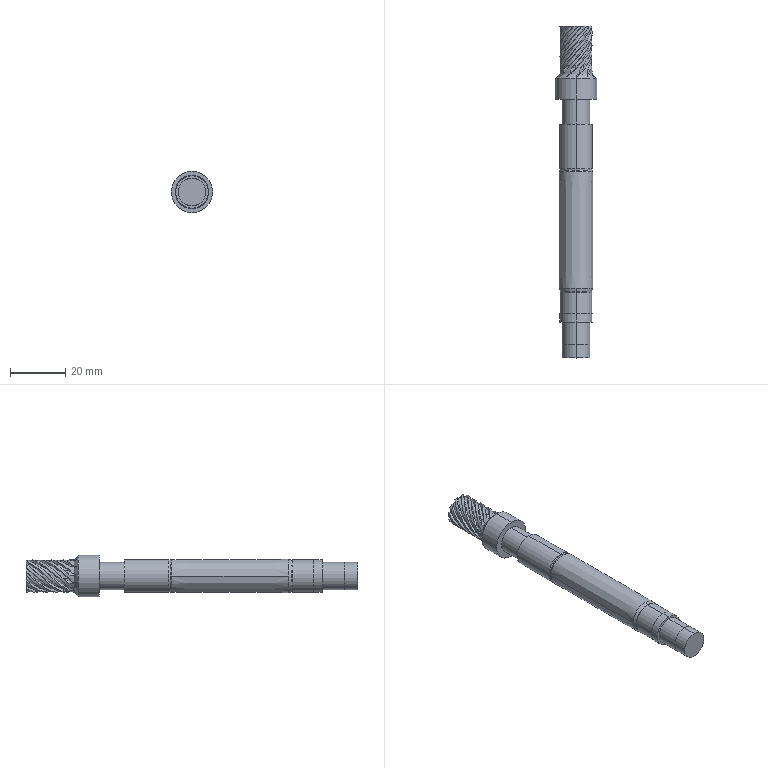Part | STEP file | 1 solid | 122 faces | box 15 x 120.2 x 15 mm | volume 12927 mm3 | spline 55 | cylinder 48 | cone 12 | plane 7 | commonest cylinder face diameters 11.6 x18 10.04 x16 10 x4 9.95 x2 11.59 x2 11.8 x2